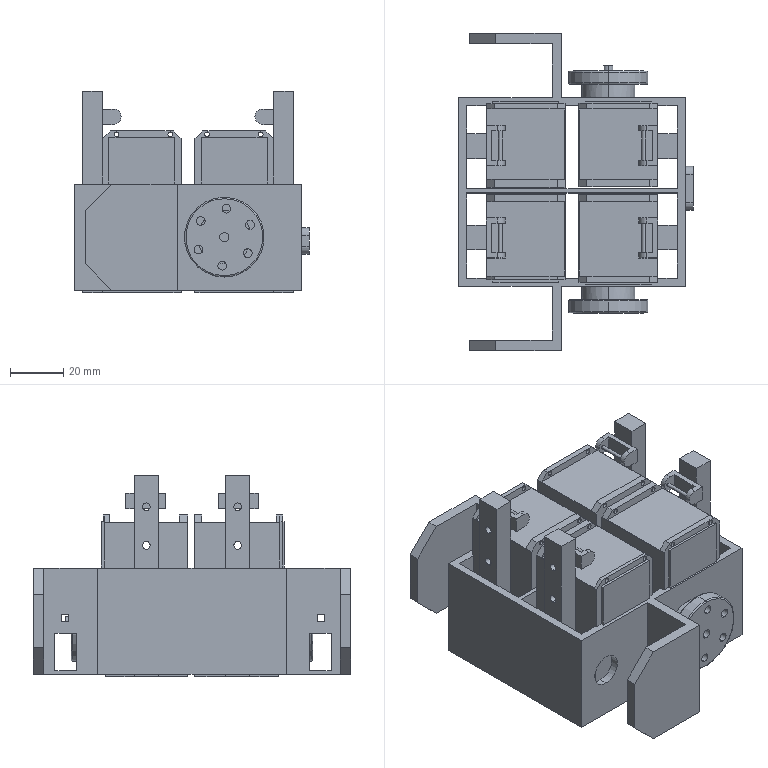Part | SolidWorks | features ICE 21, MirrorPattern 6, Fillet 5, CutThin 3, Chamfer 2, MirrorSolid 2, BossThin 1, DeleteBody 1, ExtruThin 1 | 3 solids | 374 faces | box 88.291 x 119.549 x 76 mm | volume 304358 mm3 | plane 232 | cylinder 134 | torus 8 | commonest cylinder face diameters 1.739 x32 3.288 x24 6 x24 2.864 x16 1.35 x8 3.481 x6